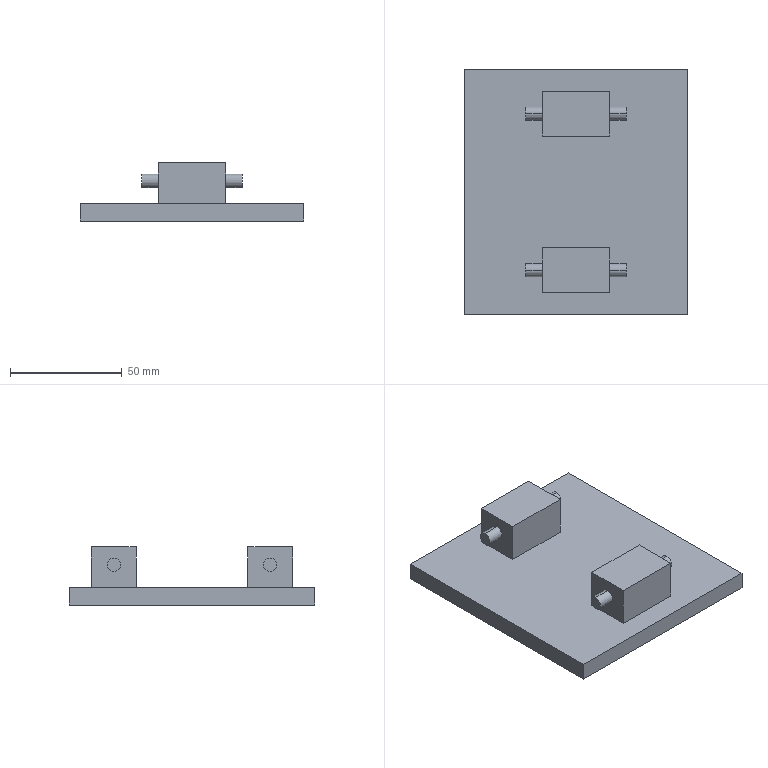Part | SolidWorks | features ICE 3, Extrusion 1 | 1 solid | 38 faces | box 100 x 110 x 26 mm | volume 81963 mm3 | plane 30 | cylinder 8 | commonest cylinder face diameters 6 x8
STEP:
#1=CARTESIAN_POINT('',(22.5,-35.,15.));
#2=VERTEX_POINT('',#1);
#3=CARTESIAN_POINT('',(22.5,-35.,21.));
#4=VERTEX_POINT('',#3);
#5=CARTESIAN_POINT('',(22.5,-35.,18.));
#6=DIRECTION('',(1.,0.,0.));
#7=DIRECTION('',(0.,0.,-1.));
#8=AXIS2_PLACEMENT_3D('',#5,#6,#7);
#9=CIRCLE('',#8,3.);
#10=EDGE_CURVE('',#2,#4,#9,.T.);
#11=ORIENTED_EDGE('',*,*,#10,.F.);
#12=CARTESIAN_POINT('',(15.,-35.,15.));
#13=VERTEX_POINT('',#12);
#14=CARTESIAN_POINT('',(22.5,-35.,15.));
#15=DIRECTION('',(-1.,0.,0.));
#16=VECTOR('',#15,1000.);
#17=LINE('',#14,#16);
#18=EDGE_CURVE('',#2,#13,#17,.T.);
#19=ORIENTED_EDGE('',*,*,#18,.T.);
#20=CARTESIAN_POINT('',(15.,-35.,21.));
#21=VERTEX_POINT('',#20);
#22=CARTESIAN_POINT('',(15.,-35.,18.));
#23=DIRECTION('',(1.,0.,0.));
#24=DIRECTION('',(0.,-1.,0.));
#25=AXIS2_PLACEMENT_3D('',#22,#23,#24);
#26=CIRCLE('',#25,3.);
#27=EDGE_CURVE('',#13,#21,#26,.T.);
#28=ORIENTED_EDGE('',*,*,#27,.T.);
#29=CARTESIAN_POINT('',(22.5,-35.,21.));
#30=DIRECTION('',(-1.,0.,0.));
#31=VECTOR('',#30,1000.);
#32=LINE('',#29,#31);
#33=EDGE_CURVE('',#4,#21,#32,.T.);
#34=ORIENTED_EDGE('',*,*,#33,.F.);
#35=EDGE_LOOP('',(#11,#19,#28,#34));
#36=FACE_OUTER_BOUND('',#35,.T.);
#37=CARTESIAN_POINT('',(22.5,-35.,18.));
#38=DIRECTION('',(-1.,0.,0.));
#39=DIRECTION('',(0.,0.,1.));
#40=AXIS2_PLACEMENT_3D('',#37,#38,#39);
#41=CYLINDRICAL_SURFACE('',#40,3.);
#42=ADVANCED_FACE('',(#36),#41,.T.);
#43=CARTESIAN_POINT('',(-15.,-35.,21.));
#44=VERTEX_POINT('',#43);
#45=CARTESIAN_POINT('',(-15.,-35.,15.));
#46=VERTEX_POINT('',#45);
#47=CARTESIAN_POINT('',(-15.,-35.,18.));
#48=DIRECTION('',(-1.,0.,0.));
#49=DIRECTION('',(0.,1.,0.));
#50=AXIS2_PLACEMENT_3D('',#47,#48,#49);
#51=CIRCLE('',#50,3.);
#52=EDGE_CURVE('',#44,#46,#51,.T.);
#53=ORIENTED_EDGE('',*,*,#52,.T.);
#54=CARTESIAN_POINT('',(-22.5,-35.,15.));
#55=VERTEX_POINT('',#54);
#56=CARTESIAN_POINT('',(22.5,-35.,15.));
#57=DIRECTION('',(-1.,0.,0.));
#58=VECTOR('',#57,1000.);
#59=LINE('',#56,#58);
#60=EDGE_CURVE('',#46,#55,#59,.T.);
#61=ORIENTED_EDGE('',*,*,#60,.T.);
#62=CARTESIAN_POINT('',(-22.5,-35.,21.));
#63=VERTEX_POINT('',#62);
#64=CARTESIAN_POINT('',(-22.5,-35.,18.));
#65=DIRECTION('',(1.,0.,0.));
#66=DIRECTION('',(0.,0.,-1.));
#67=AXIS2_PLACEMENT_3D('',#64,#65,#66);
#68=CIRCLE('',#67,3.);
#69=EDGE_CURVE('',#55,#63,#68,.T.);
#70=ORIENTED_EDGE('',*,*,#69,.T.);
#71=CARTESIAN_POINT('',(22.5,-35.,21.));
#72=DIRECTION('',(-1.,0.,0.));
#73=VECTOR('',#72,1000.);
#74=LINE('',#71,#73);
#75=EDGE_CURVE('',#44,#63,#74,.T.);
#76=ORIENTED_EDGE('',*,*,#75,.F.);
#77=EDGE_LOOP('',(#53,#61,#70,#76));
#78=FACE_OUTER_BOUND('',#77,.T.);
#79=CARTESIAN_POINT('',(22.5,-35.,18.));
#80=DIRECTION('',(-1.,0.,0.));
#81=DIRECTION('',(0.,0.,1.));
#82=AXIS2_PLACEMENT_3D('',#79,#80,#81);
#83=CYLINDRICAL_SURFACE('',#82,3.);
#84=ADVANCED_FACE('',(#78),#83,.T.);
#85=CARTESIAN_POINT('',(22.5,35.,15.));
#86=VERTEX_POINT('',#85);
#87=CARTESIAN_POINT('',(22.5,35.,21.));
#88=VERTEX_POINT('',#87);
#89=CARTESIAN_POINT('',(22.5,35.,18.));
#90=DIRECTION('',(1.,0.,0.));
#91=DIRECTION('',(0.,0.,-1.));
#92=AXIS2_PLACEMENT_3D('',#89,#90,#91);
#93=CIRCLE('',#92,3.);
#94=EDGE_CURVE('',#86,#88,#93,.T.);
#95=ORIENTED_EDGE('',*,*,#94,.F.);
#96=CARTESIAN_POINT('',(15.,35.,15.));
#97=VERTEX_POINT('',#96);
#98=CARTESIAN_POINT('',(22.5,35.,15.));
#99=DIRECTION('',(-1.,0.,0.));
#100=VECTOR('',#99,1000.);
#101=LINE('',#98,#100);
#102=EDGE_CURVE('',#86,#97,#101,.T.);
#103=ORIENTED_EDGE('',*,*,#102,.T.);
#104=CARTESIAN_POINT('',(15.,35.,21.));
#105=VERTEX_POINT('',#104);
#106=CARTESIAN_POINT('',(15.,35.,18.));
#107=DIRECTION('',(1.,0.,0.));
#108=DIRECTION('',(0.,0.,1.));
#109=AXIS2_PLACEMENT_3D('',#106,#107,#108);
#110=CIRCLE('',#109,3.);
#111=EDGE_CURVE('',#97,#105,#110,.T.);
#112=ORIENTED_EDGE('',*,*,#111,.T.);
#113=CARTESIAN_POINT('',(22.5,35.,21.));
#114=DIRECTION('',(-1.,0.,0.));
#115=VECTOR('',#114,1000.);
#116=LINE('',#113,#115);
#117=EDGE_CURVE('',#88,#105,#116,.T.);
#118=ORIENTED_EDGE('',*,*,#117,.F.);
#119=EDGE_LOOP('',(#95,#103,#112,#118));
#120=FACE_OUTER_BOUND('',#119,.T.);
#121=CARTESIAN_POINT('',(22.5,35.,18.));
#122=DIRECTION('',(-1.,0.,0.));
#123=DIRECTION('',(0.,0.,1.));
#124=AXIS2_PLACEMENT_3D('',#121,#122,#123);
#125=CYLINDRICAL_SURFACE('',#124,3.);
#126=ADVANCED_FACE('',(#120),#125,.T.);
#127=CARTESIAN_POINT('',(-15.,35.,21.));
#128=VERTEX_POINT('',#127);
#129=CARTESIAN_POINT('',(-15.,35.,15.));
#130=VERTEX_POINT('',#129);
#131=CARTESIAN_POINT('',(-15.,35.,18.));
#132=DIRECTION('',(-1.,0.,0.));
#133=DIRECTION('',(0.,0.,-1.));
#134=AXIS2_PLACEMENT_3D('',#131,#132,#133);
#135=CIRCLE('',#134,3.);
#136=EDGE_CURVE('',#128,#130,#135,.T.);
#137=ORIENTED_EDGE('',*,*,#136,.T.);
#138=CARTESIAN_POINT('',(-22.5,35.,15.));
#139=VERTEX_POINT('',#138);
#140=CARTESIAN_POINT('',(22.5,35.,15.));
#141=DIRECTION('',(-1.,0.,0.));
#142=VECTOR('',#141,1000.);
#143=LINE('',#140,#142);
#144=EDGE_CURVE('',#130,#139,#143,.T.);
#145=ORIENTED_EDGE('',*,*,#144,.T.);
#146=CARTESIAN_POINT('',(-22.5,35.,21.));
#147=VERTEX_POINT('',#146);
#148=CARTESIAN_POINT('',(-22.5,35.,18.));
#149=DIRECTION('',(1.,0.,0.));
#150=DIRECTION('',(0.,0.,-1.));
#151=AXIS2_PLACEMENT_3D('',#148,#149,#150);
#152=CIRCLE('',#151,3.);
#153=EDGE_CURVE('',#139,#147,#152,.T.);
#154=ORIENTED_EDGE('',*,*,#153,.T.);
#155=CARTESIAN_POINT('',(22.5,35.,21.));
#156=DIRECTION('',(-1.,0.,0.));
#157=VECTOR('',#156,1000.);
#158=LINE('',#155,#157);
#159=EDGE_CURVE('',#128,#147,#158,.T.);
#160=ORIENTED_EDGE('',*,*,#159,.F.);
#161=EDGE_LOOP('',(#137,#145,#154,#160));
#162=FACE_OUTER_BOUND('',#161,.T.);
#163=CARTESIAN_POINT('',(22.5,35.,18.));
#164=DIRECTION('',(-1.,0.,0.));
#165=DIRECTION('',(0.,0.,1.));
#166=AXIS2_PLACEMENT_3D('',#163,#164,#165);
#167=CYLINDRICAL_SURFACE('',#166,3.);
#168=ADVANCED_FACE('',(#162),#167,.T.);
#169=CARTESIAN_POINT('',(50.,-55.,8.));
#170=VERTEX_POINT('',#169);
#171=CARTESIAN_POINT('',(50.,55.,8.));
#172=VERTEX_POINT('',#171);
#173=CARTESIAN_POINT('',(50.,55.,8.));
#174=DIRECTION('',(0.,1.,0.));
#175=VECTOR('',#174,1000.);
#176=LINE('',#173,#175);
#177=EDGE_CURVE('',#170,#172,#176,.T.);
#178=ORIENTED_EDGE('',*,*,#177,.T.);
#179=CARTESIAN_POINT('',(-50.,55.,8.));
#180=VERTEX_POINT('',#179);
#181=CARTESIAN_POINT('',(-50.,55.,8.));
#182=DIRECTION('',(-1.,0.,0.));
#183=VECTOR('',#182,1000.);
#184=LINE('',#181,#183);
#185=EDGE_CURVE('',#172,#180,#184,.T.);
#186=ORIENTED_EDGE('',*,*,#185,.T.);
#187=CARTESIAN_POINT('',(-50.,-55.,8.));
#188=VERTEX_POINT('',#187);
#189=CARTESIAN_POINT('',(-50.,55.,8.));
#190=DIRECTION('',(0.,-1.,0.));
#191=VECTOR('',#190,1000.);
#192=LINE('',#189,#191);
#193=EDGE_CURVE('',#180,#188,#192,.T.);
#194=ORIENTED_EDGE('',*,*,#193,.T.);
#195=CARTESIAN_POINT('',(-50.,-55.,8.));
#196=DIRECTION('',(1.,0.,0.));
#197=VECTOR('',#196,1000.);
#198=LINE('',#195,#197);
#199=EDGE_CURVE('',#188,#170,#198,.T.);
#200=ORIENTED_EDGE('',*,*,#199,.T.);
#201=EDGE_LOOP('',(#178,#186,#194,#200));
#202=FACE_OUTER_BOUND('',#201,.T.);
#203=CARTESIAN_POINT('',(15.,-25.,8.));
#204=VERTEX_POINT('',#203);
#205=CARTESIAN_POINT('',(-15.,-25.,8.));
#206=VERTEX_POINT('',#205);
#207=CARTESIAN_POINT('',(-15.,-25.,8.));
#208=DIRECTION('',(-1.,0.,0.));
#209=VECTOR('',#208,1000.);
#210=LINE('',#207,#209);
#211=EDGE_CURVE('',#204,#206,#210,.T.);
#212=ORIENTED_EDGE('',*,*,#211,.F.);
#213=CARTESIAN_POINT('',(15.,-45.,8.));
#214=VERTEX_POINT('',#213);
#215=CARTESIAN_POINT('',(15.,-25.,8.));
#216=DIRECTION('',(0.,1.,0.));
#217=VECTOR('',#216,1000.);
#218=LINE('',#215,#217);
#219=EDGE_CURVE('',#214,#204,#218,.T.);
#220=ORIENTED_EDGE('',*,*,#219,.F.);
#221=CARTESIAN_POINT('',(-15.,-45.,8.));
#222=VERTEX_POINT('',#221);
#223=CARTESIAN_POINT('',(-15.,-45.,8.));
#224=DIRECTION('',(1.,0.,0.));
#225=VECTOR('',#224,1000.);
#226=LINE('',#223,#225);
#227=EDGE_CURVE('',#222,#214,#226,.T.);
#228=ORIENTED_EDGE('',*,*,#227,.F.);
#229=CARTESIAN_POINT('',(-15.,-25.,8.));
#230=DIRECTION('',(0.,-1.,0.));
#231=VECTOR('',#230,1000.);
#232=LINE('',#229,#231);
#233=EDGE_CURVE('',#206,#222,#232,.T.);
#234=ORIENTED_EDGE('',*,*,#233,.F.);
#235=EDGE_LOOP('',(#212,#220,#228,#234));
#236=FACE_BOUND('',#235,.T.);
#237=CARTESIAN_POINT('',(15.,45.,8.));
#238=VERTEX_POINT('',#237);
#239=CARTESIAN_POINT('',(-15.,45.,8.));
#240=VERTEX_POINT('',#239);
#241=CARTESIAN_POINT('',(-15.,45.,8.));
#242=DIRECTION('',(-1.,0.,0.));
#243=VECTOR('',#242,1000.);
#244=LINE('',#241,#243);
#245=EDGE_CURVE('',#238,#240,#244,.T.);
#246=ORIENTED_EDGE('',*,*,#245,.F.);
#247=CARTESIAN_POINT('',(15.,25.,8.));
#248=VERTEX_POINT('',#247);
#249=CARTESIAN_POINT('',(15.,25.,8.));
#250=DIRECTION('',(0.,1.,0.));
#251=VECTOR('',#250,1000.);
#252=LINE('',#249,#251);
#253=EDGE_CURVE('',#248,#238,#252,.T.);
#254=ORIENTED_EDGE('',*,*,#253,.F.);
#255=CARTESIAN_POINT('',(-15.,25.,8.));
#256=VERTEX_POINT('',#255);
#257=CARTESIAN_POINT('',(-15.,25.,8.));
#258=DIRECTION('',(1.,0.,0.));
#259=VECTOR('',#258,1000.);
#260=LINE('',#257,#259);
#261=EDGE_CURVE('',#256,#248,#260,.T.);
#262=ORIENTED_EDGE('',*,*,#261,.F.);
#263=CARTESIAN_POINT('',(-15.,25.,8.));
#264=DIRECTION('',(0.,-1.,0.));
#265=VECTOR('',#264,1000.);
#266=LINE('',#263,#265);
#267=EDGE_CURVE('',#240,#256,#266,.T.);
#268=ORIENTED_EDGE('',*,*,#267,.F.);
#269=EDGE_LOOP('',(#246,#254,#262,#268));
#270=FACE_BOUND('',#269,.T.);
#271=CARTESIAN_POINT('',(0.,0.,8.));
#272=DIRECTION('',(0.,0.,1.));
#273=DIRECTION('',(1.,0.,0.));
#274=AXIS2_PLACEMENT_3D('',#271,#272,#273);
#275=PLANE('',#274);
#276=ADVANCED_FACE('',(#202,#236,#270),#275,.T.);
#277=CARTESIAN_POINT('',(50.,-55.,0.));
#278=VERTEX_POINT('',#277);
#279=CARTESIAN_POINT('',(50.,55.,0.));
#280=VERTEX_POINT('',#279);
#281=CARTESIAN_POINT('',(50.,55.,0.));
#282=DIRECTION('',(0.,1.,0.));
#283=VECTOR('',#282,1000.);
#284=LINE('',#281,#283);
#285=EDGE_CURVE('',#278,#280,#284,.T.);
#286=ORIENTED_EDGE('',*,*,#285,.T.);
#287=CARTESIAN_POINT('',(50.,55.,8.));
#288=DIRECTION('',(0.,0.,-1.));
#289=VECTOR('',#288,1000.);
#290=LINE('',#287,#289);
#291=EDGE_CURVE('',#172,#280,#290,.T.);
#292=ORIENTED_EDGE('',*,*,#291,.F.);
#293=ORIENTED_EDGE('',*,*,#177,.F.);
#294=CARTESIAN_POINT('',(50.,-55.,8.));
#295=DIRECTION('',(0.,0.,-1.));
#296=VECTOR('',#295,1000.);
#297=LINE('',#294,#296);
#298=EDGE_CURVE('',#170,#278,#297,.T.);
#299=ORIENTED_EDGE('',*,*,#298,.T.);
#300=EDGE_LOOP('',(#286,#292,#293,#299));
#301=FACE_OUTER_BOUND('',#300,.T.);
#302=CARTESIAN_POINT('',(50.,55.,8.));
#303=DIRECTION('',(-1.,0.,0.));
#304=DIRECTION('',(0.,-1.,0.));
#305=AXIS2_PLACEMENT_3D('',#302,#303,#304);
#306=PLANE('',#305);
#307=ADVANCED_FACE('',(#301),#306,.F.);
#308=CARTESIAN_POINT('',(-50.,55.,0.));
#309=VERTEX_POINT('',#308);
#310=CARTESIAN_POINT('',(-50.,55.,0.));
#311=DIRECTION('',(-1.,0.,0.));
#312=VECTOR('',#311,1000.);
#313=LINE('',#310,#312);
#314=EDGE_CURVE('',#280,#309,#313,.T.);
#315=ORIENTED_EDGE('',*,*,#314,.T.);
#316=CARTESIAN_POINT('',(-50.,55.,8.));
#317=DIRECTION('',(0.,0.,-1.));
#318=VECTOR('',#317,1000.);
#319=LINE('',#316,#318);
#320=EDGE_CURVE('',#180,#309,#319,.T.);
#321=ORIENTED_EDGE('',*,*,#320,.F.);
#322=ORIENTED_EDGE('',*,*,#185,.F.);
#323=ORIENTED_EDGE('',*,*,#291,.T.);
#324=EDGE_LOOP('',(#315,#321,#322,#323));
#325=FACE_OUTER_BOUND('',#324,.T.);
#326=CARTESIAN_POINT('',(-50.,55.,8.));
#327=DIRECTION('',(0.,-1.,0.));
#328=DIRECTION('',(0.,0.,-1.));
#329=AXIS2_PLACEMENT_3D('',#326,#327,#328);
#330=PLANE('',#329);
#331=ADVANCED_FACE('',(#325),#330,.F.);
#332=CARTESIAN_POINT('',(-50.,-55.,0.));
#333=VERTEX_POINT('',#332);
#334=CARTESIAN_POINT('',(-50.,55.,0.));
#335=DIRECTION('',(0.,-1.,0.));
#336=VECTOR('',#335,1000.);
#337=LINE('',#334,#336);
#338=EDGE_CURVE('',#309,#333,#337,.T.);
#339=ORIENTED_EDGE('',*,*,#338,.T.);
#340=CARTESIAN_POINT('',(-50.,-55.,8.));
#341=DIRECTION('',(0.,0.,-1.));
#342=VECTOR('',#341,1000.);
#343=LINE('',#340,#342);
#344=EDGE_CURVE('',#188,#333,#343,.T.);
#345=ORIENTED_EDGE('',*,*,#344,.F.);
#346=ORIENTED_EDGE('',*,*,#193,.F.);
#347=ORIENTED_EDGE('',*,*,#320,.T.);
#348=EDGE_LOOP('',(#339,#345,#346,#347));
#349=FACE_OUTER_BOUND('',#348,.T.);
#350=CARTESIAN_POINT('',(-50.,55.,8.));
#351=DIRECTION('',(1.,0.,0.));
#352=DIRECTION('',(0.,1.,0.));
#353=AXIS2_PLACEMENT_3D('',#350,#351,#352);
#354=PLANE('',#353);
#355=ADVANCED_FACE('',(#349),#354,.F.);
#356=CARTESIAN_POINT('',(-50.,-55.,0.));
#357=DIRECTION('',(1.,0.,0.));
#358=VECTOR('',#357,1000.);
#359=LINE('',#356,#358);
#360=EDGE_CURVE('',#333,#278,#359,.T.);
#361=ORIENTED_EDGE('',*,*,#360,.T.);
#362=ORIENTED_EDGE('',*,*,#298,.F.);
#363=ORIENTED_EDGE('',*,*,#199,.F.);
#364=ORIENTED_EDGE('',*,*,#344,.T.);
#365=EDGE_LOOP('',(#361,#362,#363,#364));
#366=FACE_OUTER_BOUND('',#365,.T.);
#367=CARTESIAN_POINT('',(-50.,-55.,8.));
#368=DIRECTION('',(0.,1.,0.));
#369=DIRECTION('',(0.,0.,1.));
#370=AXIS2_PLACEMENT_3D('',#367,#368,#369);
#371=PLANE('',#370);
#372=ADVANCED_FACE('',(#366),#371,.F.);
#373=CARTESIAN_POINT('',(13.304,47.817,0.));
#374=VERTEX_POINT('',#373);
#375=CARTESIAN_POINT('',(42.649,47.817,0.));
#376=VERTEX_POINT('',#375);
#377=CARTESIAN_POINT('',(42.649,47.817,0.));
#378=DIRECTION('',(1.,0.,0.));
#379=VECTOR('',#378,1000.);
#380=LINE('',#377,#379);
#381=EDGE_CURVE('',#374,#376,#380,.T.);
#382=ORIENTED_EDGE('',*,*,#381,.F.);
#383=CARTESIAN_POINT('',(13.304,-43.751,0.));
#384=VERTEX_POINT('',#383);
#385=CARTESIAN_POINT('',(13.304,47.817,0.));
#386=DIRECTION('',(0.,1.,0.));
#387=VECTOR('',#386,1000.);
#388=LINE('',#385,#387);
#389=EDGE_CURVE('',#384,#374,#388,.T.);
#390=ORIENTED_EDGE('',*,*,#389,.F.);
#391=CARTESIAN_POINT('',(42.649,-43.751,0.));
#392=VERTEX_POINT('',#391);
#393=CARTESIAN_POINT('',(42.649,-43.751,0.));
#394=DIRECTION('',(-1.,0.,0.));
#395=VECTOR('',#394,1000.);
#396=LINE('',#393,#395);
#397=EDGE_CURVE('',#392,#384,#396,.T.);
#398=ORIENTED_EDGE('',*,*,#397,.F.);
#399=CARTESIAN_POINT('',(42.649,47.817,0.));
#400=DIRECTION('',(0.,-1.,0.));
#401=VECTOR('',#400,1000.);
#402=LINE('',#399,#401);
#403=EDGE_CURVE('',#376,#392,#402,.T.);
#404=ORIENTED_EDGE('',*,*,#403,.F.);
#405=EDGE_LOOP('',(#382,#390,#398,#404));
#406=FACE_BOUND('',#405,.T.);
#407=CARTESIAN_POINT('',(-44.019,47.817,0.));
#408=VERTEX_POINT('',#407);
#409=CARTESIAN_POINT('',(-11.339,47.817,0.));
#410=VERTEX_POINT('',#409);
#411=CARTESIAN_POINT('',(-11.339,47.817,0.));
#412=DIRECTION('',(1.,0.,0.));
#413=VECTOR('',#412,1000.);
#414=LINE('',#411,#413);
#415=EDGE_CURVE('',#408,#410,#414,.T.);
#416=ORIENTED_EDGE('',*,*,#415,.F.);
#417=CARTESIAN_POINT('',(-44.019,-44.287,0.));
#418=VERTEX_POINT('',#417);
#419=CARTESIAN_POINT('',(-44.019,47.817,0.));
#420=DIRECTION('',(0.,1.,0.));
#421=VECTOR('',#420,1000.);
#422=LINE('',#419,#421);
#423=EDGE_CURVE('',#418,#408,#422,.T.);
#424=ORIENTED_EDGE('',*,*,#423,.F.);
#425=CARTESIAN_POINT('',(-11.339,-44.287,0.));
#426=VERTEX_POINT('',#425);
#427=CARTESIAN_POINT('',(-11.339,-44.287,0.));
#428=DIRECTION('',(-1.,0.,0.));
#429=VECTOR('',#428,1000.);
#430=LINE('',#427,#429);
#431=EDGE_CURVE('',#426,#418,#430,.T.);
#432=ORIENTED_EDGE('',*,*,#431,.F.);
#433=CARTESIAN_POINT('',(-11.339,47.817,0.));
#434=DIRECTION('',(0.,-1.,0.));
#435=VECTOR('',#434,1000.);
#436=LINE('',#433,#435);
#437=EDGE_CURVE('',#410,#426,#436,.T.);
#438=ORIENTED_EDGE('',*,*,#437,.F.);
#439=EDGE_LOOP('',(#416,#424,#432,#438));
#440=FACE_BOUND('',#439,.T.);
#441=ORIENTED_EDGE('',*,*,#285,.F.);
#442=ORIENTED_EDGE('',*,*,#360,.F.);
#443=ORIENTED_EDGE('',*,*,#338,.F.);
#444=ORIENTED_EDGE('',*,*,#314,.F.);
#445=EDGE_LOOP('',(#441,#442,#443,#444));
#446=FACE_OUTER_BOUND('',#445,.T.);
#447=CARTESIAN_POINT('',(0.,0.,0.));
#448=DIRECTION('',(0.,0.,1.));
#449=DIRECTION('',(1.,0.,0.));
#450=AXIS2_PLACEMENT_3D('',#447,#448,#449);
#451=PLANE('',#450);
#452=ADVANCED_FACE('',(#406,#440,#446),#451,.F.);
#453=CARTESIAN_POINT('',(15.,-35.,18.));
#454=DIRECTION('',(1.,0.,0.));
#455=DIRECTION('',(0.,-1.,0.));
#456=AXIS2_PLACEMENT_3D('',#453,#454,#455);
#457=CIRCLE('',#456,3.);
#458=EDGE_CURVE('',#21,#13,#457,.T.);
#459=ORIENTED_EDGE('',*,*,#458,.F.);
#460=ORIENTED_EDGE('',*,*,#27,.F.);
#461=EDGE_LOOP('',(#459,#460));
#462=FACE_BOUND('',#461,.T.);
#463=ORIENTED_EDGE('',*,*,#219,.T.);
#464=CARTESIAN_POINT('',(15.,-25.,26.));
#465=VERTEX_POINT('',#464);
#466=CARTESIAN_POINT('',(15.,-25.,26.));
#467=DIRECTION('',(0.,0.,-1.));
#468=VECTOR('',#467,1000.);
#469=LINE('',#466,#468);
#470=EDGE_CURVE('',#465,#204,#469,.T.);
#471=ORIENTED_EDGE('',*,*,#470,.F.);
#472=CARTESIAN_POINT('',(15.,-45.,26.));
#473=VERTEX_POINT('',#472);
#474=CARTESIAN_POINT('',(15.,-25.,26.));
#475=DIRECTION('',(0.,1.,0.));
#476=VECTOR('',#475,1000.);
#477=LINE('',#474,#476);
#478=EDGE_CURVE('',#473,#465,#477,.T.);
#479=ORIENTED_EDGE('',*,*,#478,.F.);
#480=CARTESIAN_POINT('',(15.,-45.,26.));
#481=DIRECTION('',(0.,0.,-1.));
#482=VECTOR('',#481,1000.);
#483=LINE('',#480,#482);
#484=EDGE_CURVE('',#473,#214,#483,.T.);
#485=ORIENTED_EDGE('',*,*,#484,.T.);
#486=EDGE_LOOP('',(#463,#471,#479,#485));
#487=FACE_OUTER_BOUND('',#486,.T.);
#488=CARTESIAN_POINT('',(15.,-25.,26.));
#489=DIRECTION('',(-1.,0.,0.));
#490=DIRECTION('',(0.,-1.,0.));
#491=AXIS2_PLACEMENT_3D('',#488,#489,#490);
#492=PLANE('',#491);
#493=ADVANCED_FACE('',(#462,#487),#492,.F.);
#494=ORIENTED_EDGE('',*,*,#211,.T.);
#495=CARTESIAN_POINT('',(-15.,-25.,26.));
#496=VERTEX_POINT('',#495);
#497=CARTESIAN_POINT('',(-15.,-25.,26.));
#498=DIRECTION('',(0.,0.,-1.));
#499=VECTOR('',#498,1000.);
#500=LINE('',#497,#499);
#501=EDGE_CURVE('',#496,#206,#500,.T.);
#502=ORIENTED_EDGE('',*,*,#501,.F.);
#503=CARTESIAN_POINT('',(-15.,-25.,26.));
#504=DIRECTION('',(-1.,0.,0.));
#505=VECTOR('',#504,1000.);
#506=LINE('',#503,#505);
#507=EDGE_CURVE('',#465,#496,#506,.T.);
#508=ORIENTED_EDGE('',*,*,#507,.F.);
#509=ORIENTED_EDGE('',*,*,#470,.T.);
#510=EDGE_LOOP('',(#494,#502,#508,#509));
#511=FACE_OUTER_BOUND('',#510,.T.);
#512=CARTESIAN_POINT('',(-15.,-25.,26.));
#513=DIRECTION('',(0.,-1.,0.));
#514=DIRECTION('',(1.,0.,0.));
#515=AXIS2_PLACEMENT_3D('',#512,#513,#514);
#516=PLANE('',#515);
#517=ADVANCED_FACE('',(#511),#516,.F.);
#518=ORIENTED_EDGE('',*,*,#52,.F.);
#519=CARTESIAN_POINT('',(-15.,-35.,18.));
#520=DIRECTION('',(-1.,0.,0.));
#521=DIRECTION('',(0.,1.,0.));
#522=AXIS2_PLACEMENT_3D('',#519,#520,#521);
#523=CIRCLE('',#522,3.);
#524=EDGE_CURVE('',#46,#44,#523,.T.);
#525=ORIENTED_EDGE('',*,*,#524,.F.);
#526=EDGE_LOOP('',(#518,#525));
#527=FACE_BOUND('',#526,.T.);
#528=ORIENTED_EDGE('',*,*,#233,.T.);
#529=CARTESIAN_POINT('',(-15.,-45.,26.));
#530=VERTEX_POINT('',#529);
#531=CARTESIAN_POINT('',(-15.,-45.,26.));
#532=DIRECTION('',(0.,0.,-1.));
#533=VECTOR('',#532,1000.);
#534=LINE('',#531,#533);
#535=EDGE_CURVE('',#530,#222,#534,.T.);
#536=ORIENTED_EDGE('',*,*,#535,.F.);
#537=CARTESIAN_POINT('',(-15.,-25.,26.));
#538=DIRECTION('',(0.,-1.,0.));
#539=VECTOR('',#538,1000.);
#540=LINE('',#537,#539);
#541=EDGE_CURVE('',#496,#530,#540,.T.);
#542=ORIENTED_EDGE('',*,*,#541,.F.);
#543=ORIENTED_EDGE('',*,*,#501,.T.);
#544=EDGE_LOOP('',(#528,#536,#542,#543));
#545=FACE_OUTER_BOUND('',#544,.T.);
#546=CARTESIAN_POINT('',(-15.,-25.,26.));
#547=DIRECTION('',(1.,0.,0.));
#548=DIRECTION('',(0.,1.,0.));
#549=AXIS2_PLACEMENT_3D('',#546,#547,#548);
#550=PLANE('',#549);
#551=ADVANCED_FACE('',(#527,#545),#550,.F.);
#552=ORIENTED_EDGE('',*,*,#227,.T.);
#553=ORIENTED_EDGE('',*,*,#484,.F.);
#554=CARTESIAN_POINT('',(-15.,-45.,26.));
#555=DIRECTION('',(1.,0.,0.));
#556=VECTOR('',#555,1000.);
#557=LINE('',#554,#556);
#558=EDGE_CURVE('',#530,#473,#557,.T.);
#559=ORIENTED_EDGE('',*,*,#558,.F.);
#560=ORIENTED_EDGE('',*,*,#535,.T.);
#561=EDGE_LOOP('',(#552,#553,#559,#560));
#562=FACE_OUTER_BOUND('',#561,.T.);
#563=CARTESIAN_POINT('',(-15.,-45.,26.));
#564=DIRECTION('',(0.,1.,0.));
#565=DIRECTION('',(0.,0.,1.));
#566=AXIS2_PLACEMENT_3D('',#563,#564,#565);
#567=PLANE('',#566);
#568=ADVANCED_FACE('',(#562),#567,.F.);
#569=ORIENTED_EDGE('',*,*,#478,.T.);
#570=ORIENTED_EDGE('',*,*,#507,.T.);
#571=ORIENTED_EDGE('',*,*,#541,.T.);
#572=ORIENTED_EDGE('',*,*,#558,.T.);
#573=EDGE_LOOP('',(#569,#570,#571,#572));
#574=FACE_OUTER_BOUND('',#573,.T.);
#575=CARTESIAN_POINT('',(0.,0.,26.));
#576=DIRECTION('',(0.,0.,1.));
#577=DIRECTION('',(1.,0.,0.));
#578=AXIS2_PLACEMENT_3D('',#575,#576,#577);
#579=PLANE('',#578);
#580=ADVANCED_FACE('',(#574),#579,.T.);
#581=CARTESIAN_POINT('',(15.,35.,18.));
#582=DIRECTION('',(1.,0.,0.));
#583=DIRECTION('',(0.,0.,1.));
#584=AXIS2_PLACEMENT_3D('',#581,#582,#583);
#585=CIRCLE('',#584,3.);
#586=EDGE_CURVE('',#105,#97,#585,.T.);
#587=ORIENTED_EDGE('',*,*,#586,.F.);
#588=ORIENTED_EDGE('',*,*,#111,.F.);
#589=EDGE_LOOP('',(#587,#588));
#590=FACE_BOUND('',#589,.T.);
#591=ORIENTED_EDGE('',*,*,#253,.T.);
#592=CARTESIAN_POINT('',(15.,45.,26.));
#593=VERTEX_POINT('',#592);
#594=CARTESIAN_POINT('',(15.,45.,26.));
#595=DIRECTION('',(0.,0.,-1.));
#596=VECTOR('',#595,1000.);
#597=LINE('',#594,#596);
#598=EDGE_CURVE('',#593,#238,#597,.T.);
#599=ORIENTED_EDGE('',*,*,#598,.F.);
#600=CARTESIAN_POINT('',(15.,25.,26.));
#601=VERTEX_POINT('',#600);
#602=CARTESIAN_POINT('',(15.,25.,26.));
#603=DIRECTION('',(0.,1.,0.));
#604=VECTOR('',#603,1000.);
#605=LINE('',#602,#604);
#606=EDGE_CURVE('',#601,#593,#605,.T.);
#607=ORIENTED_EDGE('',*,*,#606,.F.);
#608=CARTESIAN_POINT('',(15.,25.,26.));
#609=DIRECTION('',(0.,0.,-1.));
#610=VECTOR('',#609,1000.);
#611=LINE('',#608,#610);
#612=EDGE_CURVE('',#601,#248,#611,.T.);
#613=ORIENTED_EDGE('',*,*,#612,.T.);
#614=EDGE_LOOP('',(#591,#599,#607,#613));
#615=FACE_OUTER_BOUND('',#614,.T.);
#616=CARTESIAN_POINT('',(15.,25.,26.));
#617=DIRECTION('',(-1.,0.,0.));
#618=DIRECTION('',(0.,0.,1.));
#619=AXIS2_PLACEMENT_3D('',#616,#617,#618);
#620=PLANE('',#619);
#621=ADVANCED_FACE('',(#590,#615),#620,.F.);
#622=ORIENTED_EDGE('',*,*,#245,.T.);
#623=CARTESIAN_POINT('',(-15.,45.,26.));
#624=VERTEX_POINT('',#623);
#625=CARTESIAN_POINT('',(-15.,45.,26.));
#626=DIRECTION('',(0.,0.,-1.));
#627=VECTOR('',#626,1000.);
#628=LINE('',#625,#627);
#629=EDGE_CURVE('',#624,#240,#628,.T.);
#630=ORIENTED_EDGE('',*,*,#629,.F.);
#631=CARTESIAN_POINT('',(-15.,45.,26.));
#632=DIRECTION('',(-1.,0.,0.));
#633=VECTOR('',#632,1000.);
#634=LINE('',#631,#633);
#635=EDGE_CURVE('',#593,#624,#634,.T.);
#636=ORIENTED_EDGE('',*,*,#635,.F.);
#637=ORIENTED_EDGE('',*,*,#598,.T.);
#638=EDGE_LOOP('',(#622,#630,#636,#637));
#639=FACE_OUTER_BOUND('',#638,.T.);
#640=CARTESIAN_POINT('',(-15.,45.,26.));
#641=DIRECTION('',(0.,-1.,0.));
#642=DIRECTION('',(0.,0.,-1.));
#643=AXIS2_PLACEMENT_3D('',#640,#641,#642);
#644=PLANE('',#643);
#645=ADVANCED_FACE('',(#639),#644,.F.);
#646=ORIENTED_EDGE('',*,*,#136,.F.);
#647=CARTESIAN_POINT('',(-15.,35.,18.));
#648=DIRECTION('',(-1.,0.,0.));
#649=DIRECTION('',(0.,0.,-1.));
#650=AXIS2_PLACEMENT_3D('',#647,#648,#649);
#651=CIRCLE('',#650,3.);
#652=EDGE_CURVE('',#130,#128,#651,.T.);
#653=ORIENTED_EDGE('',*,*,#652,.F.);
#654=EDGE_LOOP('',(#646,#653));
#655=FACE_BOUND('',#654,.T.);
#656=ORIENTED_EDGE('',*,*,#267,.T.);
#657=CARTESIAN_POINT('',(-15.,25.,26.));
#658=VERTEX_POINT('',#657);
#659=CARTESIAN_POINT('',(-15.,25.,26.));
#660=DIRECTION('',(0.,0.,-1.));
#661=VECTOR('',#660,1000.);
#662=LINE('',#659,#661);
#663=EDGE_CURVE('',#658,#256,#662,.T.);
#664=ORIENTED_EDGE('',*,*,#663,.F.);
#665=CARTESIAN_POINT('',(-15.,25.,26.));
#666=DIRECTION('',(0.,-1.,0.));
#667=VECTOR('',#666,1000.);
#668=LINE('',#665,#667);
#669=EDGE_CURVE('',#624,#658,#668,.T.);
#670=ORIENTED_EDGE('',*,*,#669,.F.);
#671=ORIENTED_EDGE('',*,*,#629,.T.);
#672=EDGE_LOOP('',(#656,#664,#670,#671));
#673=FACE_OUTER_BOUND('',#672,.T.);
#674=CARTESIAN_POINT('',(-15.,25.,26.));
#675=DIRECTION('',(1.,0.,0.));
#676=DIRECTION('',(0.,0.,-1.));
#677=AXIS2_PLACEMENT_3D('',#674,#675,#676);
#678=PLANE('',#677);
#679=ADVANCED_FACE('',(#655,#673),#678,.F.);
#680=ORIENTED_EDGE('',*,*,#261,.T.);
#681=ORIENTED_EDGE('',*,*,#612,.F.);
#682=CARTESIAN_POINT('',(-15.,25.,26.));
#683=DIRECTION('',(1.,0.,0.));
#684=VECTOR('',#683,1000.);
#685=LINE('',#682,#684);
#686=EDGE_CURVE('',#658,#601,#685,.T.);
#687=ORIENTED_EDGE('',*,*,#686,.F.);
#688=ORIENTED_EDGE('',*,*,#663,.T.);
#689=EDGE_LOOP('',(#680,#681,#687,#688));
#690=FACE_OUTER_BOUND('',#689,.T.);
#691=CARTESIAN_POINT('',(-15.,25.,26.));
#692=DIRECTION('',(0.,1.,0.));
#693=DIRECTION('',(-1.,0.,0.));
#694=AXIS2_PLACEMENT_3D('',#691,#692,#693);
#695=PLANE('',#694);
#696=ADVANCED_FACE('',(#690),#695,.F.);
#697=ORIENTED_EDGE('',*,*,#606,.T.);
#698=ORIENTED_EDGE('',*,*,#635,.T.);
#699=ORIENTED_EDGE('',*,*,#669,.T.);
#700=ORIENTED_EDGE('',*,*,#686,.T.);
#701=EDGE_LOOP('',(#697,#698,#699,#700));
#702=FACE_OUTER_BOUND('',#701,.T.);
#703=CARTESIAN_POINT('',(0.,0.,26.));
#704=DIRECTION('',(0.,0.,-1.));
#705=DIRECTION('',(-1.,0.,0.));
#706=AXIS2_PLACEMENT_3D('',#703,#704,#705);
#707=PLANE('',#706);
#708=ADVANCED_FACE('',(#702),#707,.F.);
#709=ORIENTED_EDGE('',*,*,#423,.T.);
#710=CARTESIAN_POINT('',(-44.019,47.817,5.));
#711=VERTEX_POINT('',#710);
#712=CARTESIAN_POINT('',(-44.019,47.817,5.));
#713=DIRECTION('',(0.,0.,-1.));
#714=VECTOR('',#713,1000.);
#715=LINE('',#712,#714);
#716=EDGE_CURVE('',#711,#408,#715,.T.);
#717=ORIENTED_EDGE('',*,*,#716,.F.);
#718=CARTESIAN_POINT('',(-44.019,-44.287,5.));
#719=VERTEX_POINT('',#718);
#720=CARTESIAN_POINT('',(-44.019,47.817,5.));
#721=DIRECTION('',(0.,1.,0.));
#722=VECTOR('',#721,1000.);
#723=LINE('',#720,#722);
#724=EDGE_CURVE('',#719,#711,#723,.T.);
#725=ORIENTED_EDGE('',*,*,#724,.F.);
#726=CARTESIAN_POINT('',(-44.019,-44.287,5.));
#727=DIRECTION('',(0.,0.,-1.));
#728=VECTOR('',#727,1000.);
#729=LINE('',#726,#728);
#730=EDGE_CURVE('',#719,#418,#729,.T.);
#731=ORIENTED_EDGE('',*,*,#730,.T.);
#732=EDGE_LOOP('',(#709,#717,#725,#731));
#733=FACE_OUTER_BOUND('',#732,.T.);
#734=CARTESIAN_POINT('',(-44.019,47.817,5.));
#735=DIRECTION('',(-1.,0.,0.));
#736=DIRECTION('',(0.,-1.,0.));
#737=AXIS2_PLACEMENT_3D('',#734,#735,#736);
#738=PLANE('',#737);
#739=ADVANCED_FACE('',(#733),#738,.F.);
#740=ORIENTED_EDGE('',*,*,#431,.T.);
#741=ORIENTED_EDGE('',*,*,#730,.F.);
#742=CARTESIAN_POINT('',(-11.339,-44.287,5.));
#743=VERTEX_POINT('',#742);
#744=CARTESIAN_POINT('',(-11.339,-44.287,5.));
#745=DIRECTION('',(-1.,0.,0.));
#746=VECTOR('',#745,1000.);
#747=LINE('',#744,#746);
#748=EDGE_CURVE('',#743,#719,#747,.T.);
#749=ORIENTED_EDGE('',*,*,#748,.F.);
#750=CARTESIAN_POINT('',(-11.339,-44.287,5.));
#751=DIRECTION('',(0.,0.,-1.));
#752=VECTOR('',#751,1000.);
#753=LINE('',#750,#752);
#754=EDGE_CURVE('',#743,#426,#753,.T.);
#755=ORIENTED_EDGE('',*,*,#754,.T.);
#756=EDGE_LOOP('',(#740,#741,#749,#755));
#757=FACE_OUTER_BOUND('',#756,.T.);
#758=CARTESIAN_POINT('',(-11.339,-44.287,5.));
#759=DIRECTION('',(0.,-1.,0.));
#760=DIRECTION('',(0.,0.,-1.));
#761=AXIS2_PLACEMENT_3D('',#758,#759,#760);
#762=PLANE('',#761);
#763=ADVANCED_FACE('',(#757),#762,.F.);
#764=ORIENTED_EDGE('',*,*,#437,.T.);
#765=ORIENTED_EDGE('',*,*,#754,.F.);
#766=CARTESIAN_POINT('',(-11.339,47.817,5.));
#767=VERTEX_POINT('',#766);
#768=CARTESIAN_POINT('',(-11.339,47.817,5.));
#769=DIRECTION('',(0.,-1.,0.));
#770=VECTOR('',#769,1000.);
#771=LINE('',#768,#770);
#772=EDGE_CURVE('',#767,#743,#771,.T.);
#773=ORIENTED_EDGE('',*,*,#772,.F.);
#774=CARTESIAN_POINT('',(-11.339,47.817,5.));
#775=DIRECTION('',(0.,0.,-1.));
#776=VECTOR('',#775,1000.);
#777=LINE('',#774,#776);
#778=EDGE_CURVE('',#767,#410,#777,.T.);
#779=ORIENTED_EDGE('',*,*,#778,.T.);
#780=EDGE_LOOP('',(#764,#765,#773,#779));
#781=FACE_OUTER_BOUND('',#780,.T.);
#782=CARTESIAN_POINT('',(-11.339,47.817,5.));
#783=DIRECTION('',(1.,0.,0.));
#784=DIRECTION('',(0.,0.,-1.));
#785=AXIS2_PLACEMENT_3D('',#782,#783,#784);
#786=PLANE('',#785);
#787=ADVANCED_FACE('',(#781),#786,.F.);
#788=ORIENTED_EDGE('',*,*,#415,.T.);
#789=ORIENTED_EDGE('',*,*,#778,.F.);
#790=CARTESIAN_POINT('',(-11.339,47.817,5.));
#791=DIRECTION('',(1.,0.,0.));
#792=VECTOR('',#791,1000.);
#793=LINE('',#790,#792);
#794=EDGE_CURVE('',#711,#767,#793,.T.);
#795=ORIENTED_EDGE('',*,*,#794,.F.);
#796=ORIENTED_EDGE('',*,*,#716,.T.);
#797=EDGE_LOOP('',(#788,#789,#795,#796));
#798=FACE_OUTER_BOUND('',#797,.T.);
#799=CARTESIAN_POINT('',(-11.339,47.817,5.));
#800=DIRECTION('',(0.,1.,0.));
#801=DIRECTION('',(0.,0.,1.));
#802=AXIS2_PLACEMENT_3D('',#799,#800,#801);
#803=PLANE('',#802);
#804=ADVANCED_FACE('',(#798),#803,.F.);
#805=ORIENTED_EDGE('',*,*,#724,.T.);
#806=ORIENTED_EDGE('',*,*,#794,.T.);
#807=ORIENTED_EDGE('',*,*,#772,.T.);
#808=ORIENTED_EDGE('',*,*,#748,.T.);
#809=EDGE_LOOP('',(#805,#806,#807,#808));
#810=FACE_OUTER_BOUND('',#809,.T.);
#811=CARTESIAN_POINT('',(0.,0.,5.));
#812=DIRECTION('',(0.,0.,-1.));
#813=DIRECTION('',(-1.,0.,0.));
#814=AXIS2_PLACEMENT_3D('',#811,#812,#813);
#815=PLANE('',#814);
#816=ADVANCED_FACE('',(#810),#815,.T.);
#817=ORIENTED_EDGE('',*,*,#389,.T.);
#818=CARTESIAN_POINT('',(13.304,47.817,5.));
#819=VERTEX_POINT('',#818);
#820=CARTESIAN_POINT('',(13.304,47.817,5.));
#821=DIRECTION('',(0.,0.,-1.));
#822=VECTOR('',#821,1000.);
#823=LINE('',#820,#822);
#824=EDGE_CURVE('',#819,#374,#823,.T.);
#825=ORIENTED_EDGE('',*,*,#824,.F.);
#826=CARTESIAN_POINT('',(13.304,-43.751,5.));
#827=VERTEX_POINT('',#826);
#828=CARTESIAN_POINT('',(13.304,47.817,5.));
#829=DIRECTION('',(0.,1.,0.));
#830=VECTOR('',#829,1000.);
#831=LINE('',#828,#830);
#832=EDGE_CURVE('',#827,#819,#831,.T.);
#833=ORIENTED_EDGE('',*,*,#832,.F.);
#834=CARTESIAN_POINT('',(13.304,-43.751,5.));
#835=DIRECTION('',(0.,0.,-1.));
#836=VECTOR('',#835,1000.);
#837=LINE('',#834,#836);
#838=EDGE_CURVE('',#827,#384,#837,.T.);
#839=ORIENTED_EDGE('',*,*,#838,.T.);
#840=EDGE_LOOP('',(#817,#825,#833,#839));
#841=FACE_OUTER_BOUND('',#840,.T.);
#842=CARTESIAN_POINT('',(13.304,47.817,5.));
#843=DIRECTION('',(-1.,0.,0.));
#844=DIRECTION('',(0.,-1.,0.));
#845=AXIS2_PLACEMENT_3D('',#842,#843,#844);
#846=PLANE('',#845);
#847=ADVANCED_FACE('',(#841),#846,.F.);
#848=ORIENTED_EDGE('',*,*,#397,.T.);
#849=ORIENTED_EDGE('',*,*,#838,.F.);
#850=CARTESIAN_POINT('',(42.649,-43.751,5.));
#851=VERTEX_POINT('',#850);
#852=CARTESIAN_POINT('',(42.649,-43.751,5.));
#853=DIRECTION('',(-1.,0.,0.));
#854=VECTOR('',#853,1000.);
#855=LINE('',#852,#854);
#856=EDGE_CURVE('',#851,#827,#855,.T.);
#857=ORIENTED_EDGE('',*,*,#856,.F.);
#858=CARTESIAN_POINT('',(42.649,-43.751,5.));
#859=DIRECTION('',(0.,0.,-1.));
#860=VECTOR('',#859,1000.);
#861=LINE('',#858,#860);
#862=EDGE_CURVE('',#851,#392,#861,.T.);
#863=ORIENTED_EDGE('',*,*,#862,.T.);
#864=EDGE_LOOP('',(#848,#849,#857,#863));
#865=FACE_OUTER_BOUND('',#864,.T.);
#866=CARTESIAN_POINT('',(42.649,-43.751,5.));
#867=DIRECTION('',(0.,-1.,0.));
#868=DIRECTION('',(0.,0.,-1.));
#869=AXIS2_PLACEMENT_3D('',#866,#867,#868);
#870=PLANE('',#869);
#871=ADVANCED_FACE('',(#865),#870,.F.);
#872=ORIENTED_EDGE('',*,*,#403,.T.);
#873=ORIENTED_EDGE('',*,*,#862,.F.);
#874=CARTESIAN_POINT('',(42.649,47.817,5.));
#875=VERTEX_POINT('',#874);
#876=CARTESIAN_POINT('',(42.649,47.817,5.));
#877=DIRECTION('',(0.,-1.,0.));
#878=VECTOR('',#877,1000.);
#879=LINE('',#876,#878);
#880=EDGE_CURVE('',#875,#851,#879,.T.);
#881=ORIENTED_EDGE('',*,*,#880,.F.);
#882=CARTESIAN_POINT('',(42.649,47.817,5.));
#883=DIRECTION('',(0.,0.,-1.));
#884=VECTOR('',#883,1000.);
#885=LINE('',#882,#884);
#886=EDGE_CURVE('',#875,#376,#885,.T.);
#887=ORIENTED_EDGE('',*,*,#886,.T.);
#888=EDGE_LOOP('',(#872,#873,#881,#887));
#889=FACE_OUTER_BOUND('',#888,.T.);
#890=CARTESIAN_POINT('',(42.649,47.817,5.));
#891=DIRECTION('',(1.,0.,0.));
#892=DIRECTION('',(0.,0.,-1.));
#893=AXIS2_PLACEMENT_3D('',#890,#891,#892);
#894=PLANE('',#893);
#895=ADVANCED_FACE('',(#889),#894,.F.);
#896=ORIENTED_EDGE('',*,*,#381,.T.);
#897=ORIENTED_EDGE('',*,*,#886,.F.);
#898=CARTESIAN_POINT('',(42.649,47.817,5.));
#899=DIRECTION('',(1.,0.,0.));
#900=VECTOR('',#899,1000.);
#901=LINE('',#898,#900);
#902=EDGE_CURVE('',#819,#875,#901,.T.);
#903=ORIENTED_EDGE('',*,*,#902,.F.);
#904=ORIENTED_EDGE('',*,*,#824,.T.);
#905=EDGE_LOOP('',(#896,#897,#903,#904));
#906=FACE_OUTER_BOUND('',#905,.T.);
#907=CARTESIAN_POINT('',(42.649,47.817,5.));
#908=DIRECTION('',(0.,1.,0.));
#909=DIRECTION('',(0.,0.,1.));
#910=AXIS2_PLACEMENT_3D('',#907,#908,#909);
#911=PLANE('',#910);
#912=ADVANCED_FACE('',(#906),#911,.F.);
#913=ORIENTED_EDGE('',*,*,#832,.T.);
#914=ORIENTED_EDGE('',*,*,#902,.T.);
#915=ORIENTED_EDGE('',*,*,#880,.T.);
#916=ORIENTED_EDGE('',*,*,#856,.T.);
#917=EDGE_LOOP('',(#913,#914,#915,#916));
#918=FACE_OUTER_BOUND('',#917,.T.);
#919=CARTESIAN_POINT('',(0.,0.,5.));
#920=DIRECTION('',(0.,0.,-1.));
#921=DIRECTION('',(-1.,0.,0.));
#922=AXIS2_PLACEMENT_3D('',#919,#920,#921);
#923=PLANE('',#922);
#924=ADVANCED_FACE('',(#918),#923,.T.);
#925=CARTESIAN_POINT('',(-22.5,35.,18.));
#926=DIRECTION('',(1.,0.,0.));
#927=DIRECTION('',(0.,0.,-1.));
#928=AXIS2_PLACEMENT_3D('',#925,#926,#927);
#929=CIRCLE('',#928,3.);
#930=EDGE_CURVE('',#147,#139,#929,.T.);
#931=ORIENTED_EDGE('',*,*,#930,.F.);
#932=ORIENTED_EDGE('',*,*,#153,.F.);
#933=EDGE_LOOP('',(#931,#932));
#934=FACE_OUTER_BOUND('',#933,.T.);
#935=CARTESIAN_POINT('',(-22.5,35.,18.));
#936=DIRECTION('',(1.,0.,0.));
#937=DIRECTION('',(0.,0.,-1.));
#938=AXIS2_PLACEMENT_3D('',#935,#936,#937);
#939=PLANE('',#938);
#940=ADVANCED_FACE('',(#934),#939,.F.);
#941=ORIENTED_EDGE('',*,*,#144,.F.);
#942=ORIENTED_EDGE('',*,*,#652,.T.);
#943=ORIENTED_EDGE('',*,*,#159,.T.);
#944=ORIENTED_EDGE('',*,*,#930,.T.);
#945=EDGE_LOOP('',(#941,#942,#943,#944));
#946=FACE_OUTER_BOUND('',#945,.T.);
#947=CARTESIAN_POINT('',(22.5,35.,18.));
#948=DIRECTION('',(-1.,0.,0.));
#949=DIRECTION('',(0.,0.,1.));
#950=AXIS2_PLACEMENT_3D('',#947,#948,#949);
#951=CYLINDRICAL_SURFACE('',#950,3.);
#952=ADVANCED_FACE('',(#946),#951,.T.);
#953=ORIENTED_EDGE('',*,*,#102,.F.);
#954=CARTESIAN_POINT('',(22.5,35.,18.));
#955=DIRECTION('',(1.,0.,0.));
#956=DIRECTION('',(0.,0.,-1.));
#957=AXIS2_PLACEMENT_3D('',#954,#955,#956);
#958=CIRCLE('',#957,3.);
#959=EDGE_CURVE('',#88,#86,#958,.T.);
#960=ORIENTED_EDGE('',*,*,#959,.F.);
#961=ORIENTED_EDGE('',*,*,#117,.T.);
#962=ORIENTED_EDGE('',*,*,#586,.T.);
#963=EDGE_LOOP('',(#953,#960,#961,#962));
#964=FACE_OUTER_BOUND('',#963,.T.);
#965=CARTESIAN_POINT('',(22.5,35.,18.));
#966=DIRECTION('',(-1.,0.,0.));
#967=DIRECTION('',(0.,0.,1.));
#968=AXIS2_PLACEMENT_3D('',#965,#966,#967);
#969=CYLINDRICAL_SURFACE('',#968,3.);
#970=ADVANCED_FACE('',(#964),#969,.T.);
#971=ORIENTED_EDGE('',*,*,#959,.T.);
#972=ORIENTED_EDGE('',*,*,#94,.T.);
#973=EDGE_LOOP('',(#971,#972));
#974=FACE_OUTER_BOUND('',#973,.T.);
#975=CARTESIAN_POINT('',(22.5,35.,18.));
#976=DIRECTION('',(1.,0.,0.));
#977=DIRECTION('',(0.,0.,-1.));
#978=AXIS2_PLACEMENT_3D('',#975,#976,#977);
#979=PLANE('',#978);
#980=ADVANCED_FACE('',(#974),#979,.T.);
#981=CARTESIAN_POINT('',(-22.5,-35.,18.));
#982=DIRECTION('',(1.,0.,0.));
#983=DIRECTION('',(0.,0.,-1.));
#984=AXIS2_PLACEMENT_3D('',#981,#982,#983);
#985=CIRCLE('',#984,3.);
#986=EDGE_CURVE('',#63,#55,#985,.T.);
#987=ORIENTED_EDGE('',*,*,#986,.F.);
#988=ORIENTED_EDGE('',*,*,#69,.F.);
#989=EDGE_LOOP('',(#987,#988));
#990=FACE_OUTER_BOUND('',#989,.T.);
#991=CARTESIAN_POINT('',(-22.5,-35.,18.));
#992=DIRECTION('',(1.,0.,0.));
#993=DIRECTION('',(0.,0.,-1.));
#994=AXIS2_PLACEMENT_3D('',#991,#992,#993);
#995=PLANE('',#994);
#996=ADVANCED_FACE('',(#990),#995,.F.);
#997=ORIENTED_EDGE('',*,*,#60,.F.);
#998=ORIENTED_EDGE('',*,*,#524,.T.);
#999=ORIENTED_EDGE('',*,*,#75,.T.);
#1000=ORIENTED_EDGE('',*,*,#986,.T.);
#1001=EDGE_LOOP('',(#997,#998,#999,#1000));
#1002=FACE_OUTER_BOUND('',#1001,.T.);
#1003=CARTESIAN_POINT('',(22.5,-35.,18.));
#1004=DIRECTION('',(-1.,0.,0.));
#1005=DIRECTION('',(0.,0.,1.));
#1006=AXIS2_PLACEMENT_3D('',#1003,#1004,#1005);
#1007=CYLINDRICAL_SURFACE('',#1006,3.);
#1008=ADVANCED_FACE('',(#1002),#1007,.T.);
#1009=ORIENTED_EDGE('',*,*,#18,.F.);
#1010=CARTESIAN_POINT('',(22.5,-35.,18.));
#1011=DIRECTION('',(1.,0.,0.));
#1012=DIRECTION('',(0.,0.,-1.));
#1013=AXIS2_PLACEMENT_3D('',#1010,#1011,#1012);
#1014=CIRCLE('',#1013,3.);
#1015=EDGE_CURVE('',#4,#2,#1014,.T.);
#1016=ORIENTED_EDGE('',*,*,#1015,.F.);
#1017=ORIENTED_EDGE('',*,*,#33,.T.);
#1018=ORIENTED_EDGE('',*,*,#458,.T.);
#1019=EDGE_LOOP('',(#1009,#1016,#1017,#1018));
#1020=FACE_OUTER_BOUND('',#1019,.T.);
#1021=CARTESIAN_POINT('',(22.5,-35.,18.));
#1022=DIRECTION('',(-1.,0.,0.));
#1023=DIRECTION('',(0.,0.,1.));
#1024=AXIS2_PLACEMENT_3D('',#1021,#1022,#1023);
#1025=CYLINDRICAL_SURFACE('',#1024,3.);
#1026=ADVANCED_FACE('',(#1020),#1025,.T.);
#1027=ORIENTED_EDGE('',*,*,#1015,.T.);
#1028=ORIENTED_EDGE('',*,*,#10,.T.);
#1029=EDGE_LOOP('',(#1027,#1028));
#1030=FACE_OUTER_BOUND('',#1029,.T.);
#1031=CARTESIAN_POINT('',(22.5,-35.,18.));
#1032=DIRECTION('',(1.,0.,0.));
#1033=DIRECTION('',(0.,0.,-1.));
#1034=AXIS2_PLACEMENT_3D('',#1031,#1032,#1033);
#1035=PLANE('',#1034);
#1036=ADVANCED_FACE('',(#1030),#1035,.T.);
#1037=CLOSED_SHELL('',(#42,#84,#126,#168,#276,#307,#331,#355,#372,#452,#493,#517,#551,#568,#580,#621,#645,#679,#696,#708,#739,#763,#787,#804,#816,#847,#871,#895,#912,#924,#940,#952,#970,#980,#996,#1008,#1026,#1036));
#1038=MANIFOLD_SOLID_BREP('',#1037);
#1039=CARTESIAN_POINT('',(0.,0.,0.));
#1040=DIRECTION('',(0.,0.,1.));
#1041=DIRECTION('',(1.,0.,0.));
#1042=AXIS2_PLACEMENT_3D('',#1039,#1040,#1041);
#1043=(LENGTH_UNIT()NAMED_UNIT(*)SI_UNIT(.MILLI.,.METRE.));
#1044=UNCERTAINTY_MEASURE_WITH_UNIT(LENGTH_MEASURE(0.00001),#1043,'','');
#1045=(NAMED_UNIT(*)PLANE_ANGLE_UNIT()SI_UNIT($,.RADIAN.));
#1046=(NAMED_UNIT(*)SI_UNIT($,.STERADIAN.)SOLID_ANGLE_UNIT());
#1047=(GEOMETRIC_REPRESENTATION_CONTEXT(3)GLOBAL_UNCERTAINTY_ASSIGNED_CONTEXT((#1044))GLOBAL_UNIT_ASSIGNED_CONTEXT((#1043,#1045,#1046))REPRESENTATION_CONTEXT('',''));
#1048=ADVANCED_BREP_SHAPE_REPRESENTATION('',(#1038,#1042),#1047);